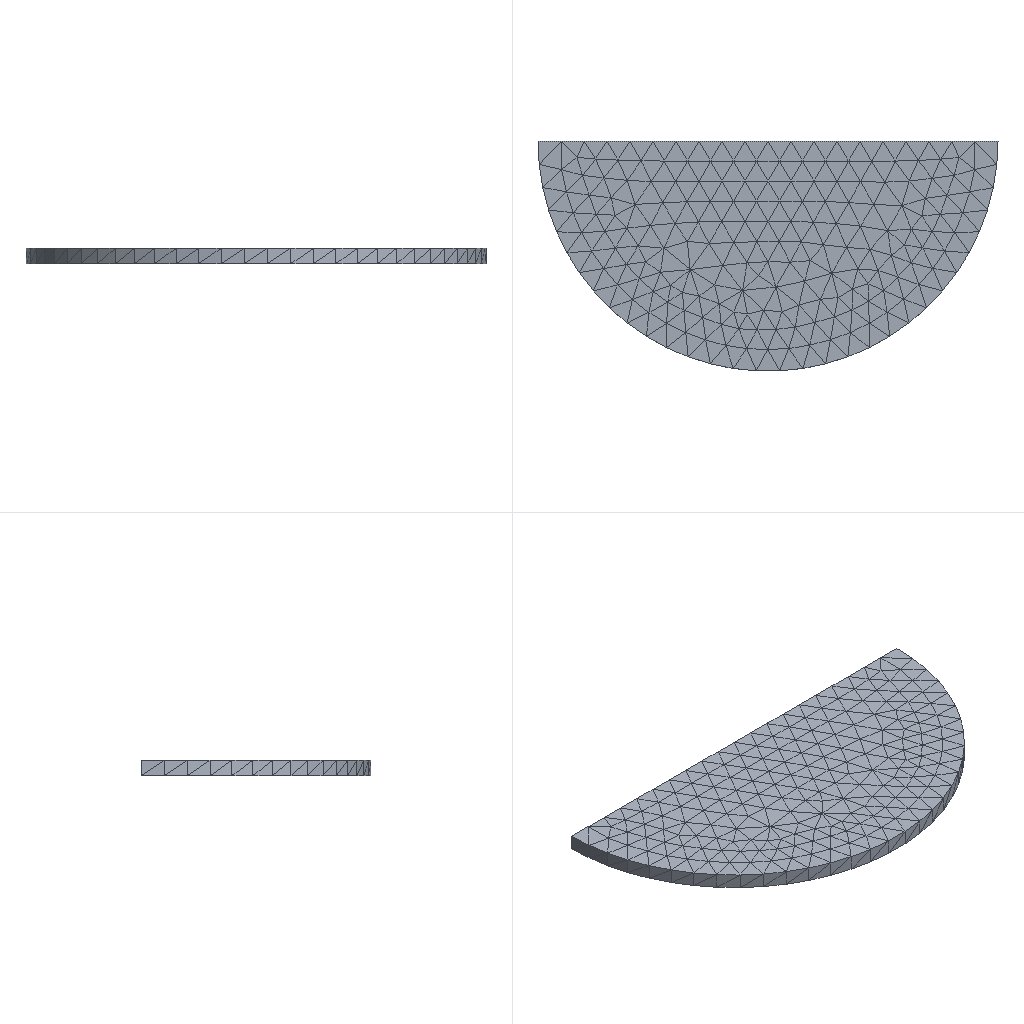Simulation study | abaqus
Notes in the study folder:
18 half-cylinder shell proxy
job_status=None
Umax_mm=5.92112e-05
S_Mises_max_MPa=0.776917
Set-up summary:
category,name,step,type,value,unit,region
solver,abaqus,,Abaqus/CAE 2024
units,mm-N-s-tonne (MPa),,inferred,E=210000 density=7.85e-09
analysis,Step-1,,static,time_period=1
mesh,nodes,,,2453
mesh,elements,,,1165
element_type,C3D10,,,1165
material,Steel,,E,210000
material,Steel,,nu,0.3
material,Steel,,density,7.85e-09
section,Steel,,solid section,,,_PickedSet2
load,Load,Step-1,pressure,0.5,,LOAD
bc,BC,Step-1,encastre,[dofs=ENCASTRE],,FIXED
Abaqus input file, long lists of numbers shortened:
*Heading
** Job name: deck Model name: M18
** Generated by: Abaqus/CAE 2024
*Preprint, echo=NO, model=NO, history=NO, contact=NO
**
** PARTS
**
*Part, name=P
*Node
      1,         -30.,           0.,           0.
      2,          30.,           0.,           0.
** (2451 more lines like these left out)
*Element, type=C3D10
   1,  265,  354,   54,  103,  436,  435,  434,  438,  437,  439
   2,  426,   73,   24,    4,  442,  441,  440,  444,  443,  445
** (1163 more lines like these left out)
*Nset, nset=_PickedSet2, internal, generate
    1,  2453,     1
*Elset, elset=_PickedSet2, internal, generate
    1,  1165,     1
** Section: Sec
*Solid Section, elset=_PickedSet2, material=Steel
,
*End Part
**
**
** ASSEMBLY
**
*Assembly, name=Assembly
**
*Instance, name=I, part=P
*End Instance
**
*Nset, nset=FIXED, instance=I
    1,    2,    3,    4,    5,    6,    7,    8,    9,   10,   11,   12,   13,   14,   15,   16
   17,   18,   19,   20,   21,   22,   23,   54,   55,   56,   57,   58,   59,   60,   61,   62
** (6 more lines like these left out)
*Elset, elset=FIXED, instance=I
    7,  123,  130,  299,  346,  404,  492,  577,  592,  608,  620,  646,  661,  693,  702,  703
  708,  710,  733,  735,  739,  741,  746,  751,  904,  908,  934,  967, 1026, 1028, 1062, 1064
** (1 more lines like these left out)
*Elset, elset=_LOAD_S3, internal, instance=I
    2,    4,   21,  253,  268,  359,  386,  388,  452,  506,  553,  559,  611,  630,  636,  657
  658,  664,  667,  674,  685,  835,  902,  906,  991, 1000, 1019, 1042, 1078, 1119, 1127, 1141
*Elset, elset=_LOAD_S4, internal, instance=I
  201,  206,  258,  261,  291,  295,  355,  371,  623,  637,  641,  654,  671,  871,  917,  937
 1110, 1139
*Elset, elset=_LOAD_S2, internal, instance=I
  612,  655, 1009, 1037, 1151
*Elset, elset=_LOAD_S1, internal, instance=I
  614,  615,  863,  878, 1010, 1152, 1154
*Surface, type=ELEMENT, name=LOAD
_LOAD_S3, S3
_LOAD_S4, S4
_LOAD_S2, S2
_LOAD_S1, S1
*End Assembly
**
** MATERIALS
**
*Material, name=Steel
*Density
 7.85e-09,
*Elastic
210000., 0.3
** ----------------------------------------------------------------
**
** STEP: Step-1
**
*Step, name=Step-1, nlgeom=NO
*Static
1., 1., 1e-05, 1.
**
** BOUNDARY CONDITIONS
**
** Name: BC Type: Symmetry/Antisymmetry/Encastre
*Boundary
FIXED, ENCASTRE
**
** LOADS
**
** Name: Load   Type: Pressure
*Dsload
LOAD, P, 0.5
**
** OUTPUT REQUESTS
**
*Restart, write, frequency=0
**
** FIELD OUTPUT: F-Output-1
**
*Output, field, variable=PRESELECT
**
** HISTORY OUTPUT: H-Output-1
**
*Output, history, variable=PRESELECT
*End Step
Results summary:
result,odb.job_status,,,JOB_STATUS_COMPLETED_SUCCESSFULLY,"consistent, unstated (Abaqus has no unit system)"
result,steps[0].procedure,Step-1,,*STATIC,"consistent, unstated (Abaqus has no unit system)"
result,steps[0].time_period,Step-1,,1,"consistent, unstated (Abaqus has no unit system)"
result,steps[0].n_frames,Step-1,,2,"consistent, unstated (Abaqus has no unit system)"
result,steps[0].last_frame.id,Step-1,,1,"consistent, unstated (Abaqus has no unit system)"
result,steps[0].last_frame.value,Step-1,,1,"consistent, unstated (Abaqus has no unit system)"
result,steps[0].last_frame.description,Step-1,,Increment      1: Step Time =    1.000,"consistent, unstated (Abaqus has no unit system)"
result,steps[0].completed,Step-1,,True,"consistent, unstated (Abaqus has no unit system)"
result,steps[0].max_U_magnitude,Step-1,,5.92112e-05,"consistent, unstated (Abaqus has no unit system)"
result,steps[0].max_S_mises,Step-1,,0.7769,"consistent, unstated (Abaqus has no unit system)"
result,steps[0].RF_sum[1],Step-1,,-4.54485e-07,"consistent, unstated (Abaqus has no unit system)"
result,steps[0].RF_sum[2],Step-1,,-60,"consistent, unstated (Abaqus has no unit system)"
result,steps[0].RF_sum[3],Step-1,,2.08616e-07,"consistent, unstated (Abaqus has no unit system)"
result,steps[1].procedure,Step-1,,*STATIC,"consistent, unstated (Abaqus has no unit system)"
result,steps[1].time_period,Step-1,,1,"consistent, unstated (Abaqus has no unit system)"
result,steps[1].n_frames,Step-1,,2,"consistent, unstated (Abaqus has no unit system)"
result,steps[1].last_frame.id,Step-1,,1,"consistent, unstated (Abaqus has no unit system)"
result,steps[1].last_frame.value,Step-1,,1,"consistent, unstated (Abaqus has no unit system)"
result,steps[1].last_frame.description,Step-1,,Increment      1: Step Time =    1.000,"consistent, unstated (Abaqus has no unit system)"
result,steps[1].completed,Step-1,,True,"consistent, unstated (Abaqus has no unit system)"
result,steps[1].max_U_magnitude,Step-1,,5.92112e-05,"consistent, unstated (Abaqus has no unit system)"
result,steps[1].max_S_mises,Step-1,,0.7769,"consistent, unstated (Abaqus has no unit system)"
result,steps[1].RF_sum[1],Step-1,,-4.54485e-07,"consistent, unstated (Abaqus has no unit system)"
result,steps[1].RF_sum[2],Step-1,,-60,"consistent, unstated (Abaqus has no unit system)"
result,steps[1].RF_sum[3],Step-1,,2.08616e-07,"consistent, unstated (Abaqus has no unit system)"